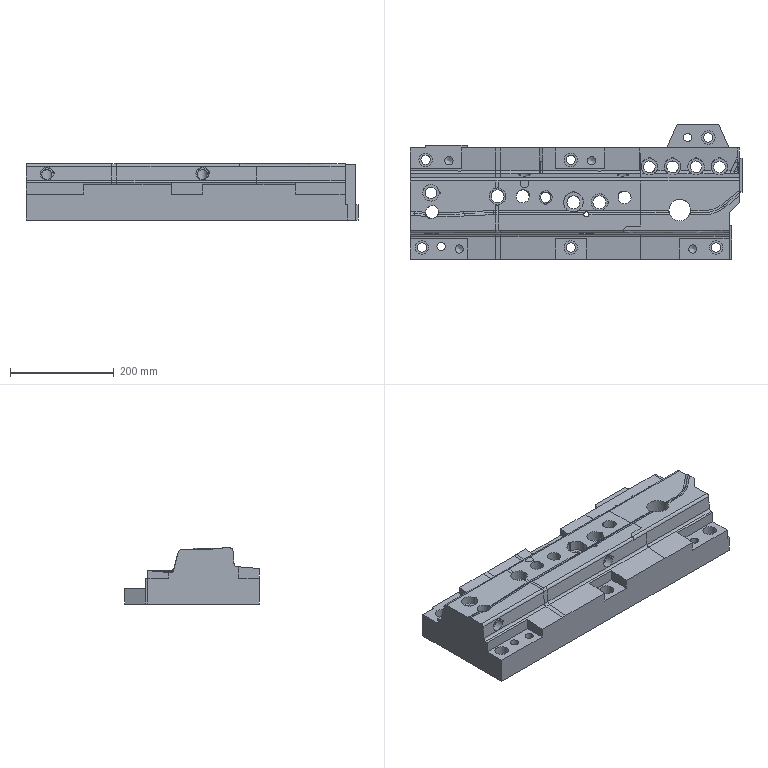Part | NX | features solid 2 | 1 solid | 231 faces | box 640 x 260 x 108.199 mm | volume 8623447 mm3 | plane 84 | cylinder 81 | spline 61 | cone 4 | torus 1 | commonest cylinder face diameters 4 x13 25 x9 10 x8 18 x8 32 x7 12 x6